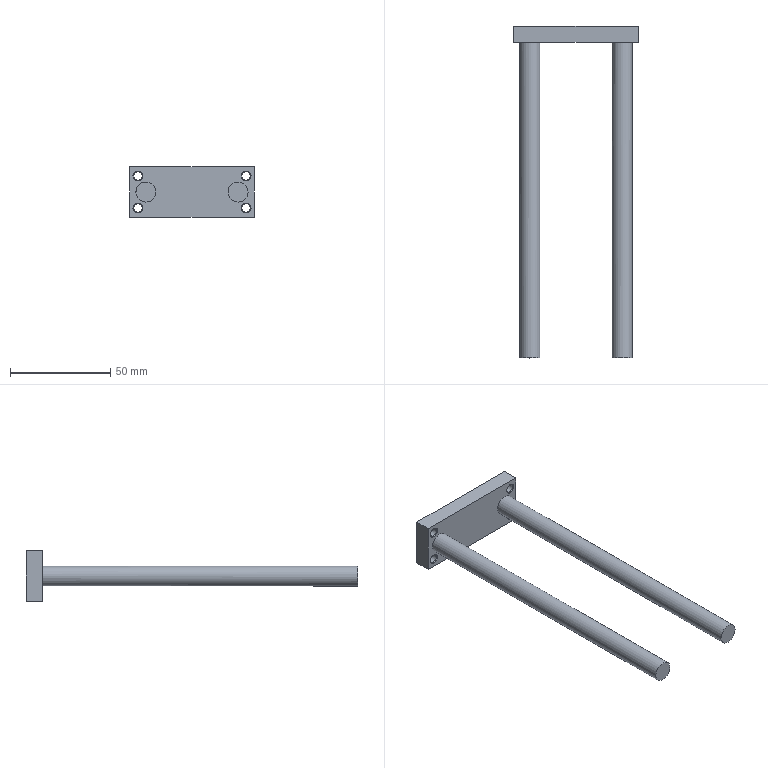Part | STEP file | Tube feed_id878_x_t | 1 solid | 22 faces | box 62 x 165.8 x 25 mm | volume 36735 mm3 | plane 8 | cone 8 | cylinder 6 | commonest cylinder face diameters 4.2 x4 10 x2